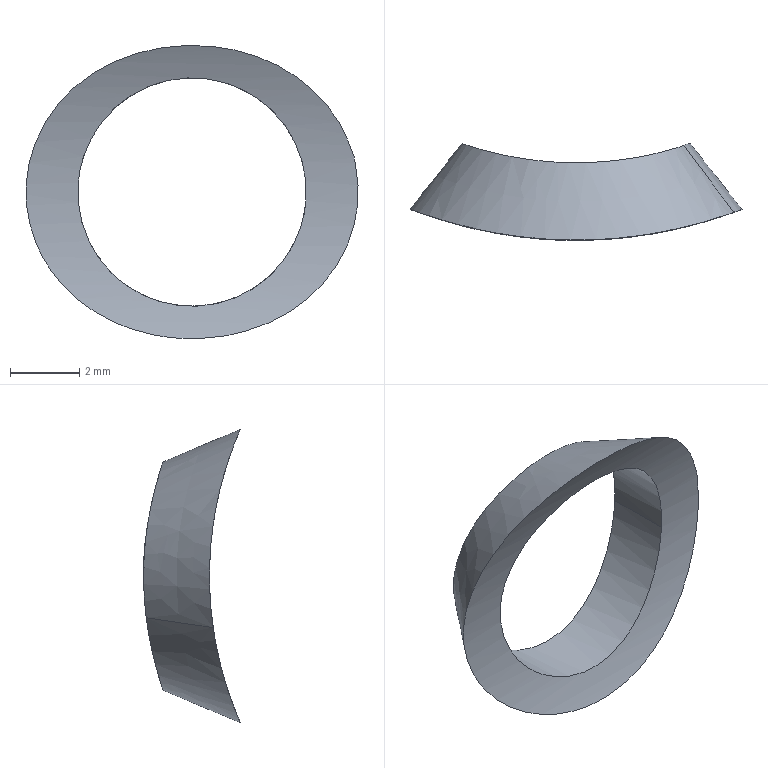Part | STEP file | 2026.6.15-Main Assembly图.sldasm-Part-181 | 1 solid | 5 faces | box 9.599 x 2.798 x 8.476 mm | volume 26.852 mm3 | cylinder 3 | spline 2 | commonest cylinder face diameters 6.6 x2 21 x1
STEP:
#1=CARTESIAN_POINT('',(-1619.46,1436.593,3406.881));
#2=VERTEX_POINT('',#1);
#3=CARTESIAN_POINT('',(-1620.893,1434.658,3406.596));
#4=VERTEX_POINT('',#3);
#5=CARTESIAN_POINT('',(-1619.46,1436.593,3406.881));
#6=CARTESIAN_POINT('',(-1620.893,1434.658,3406.596));
#7=B_SPLINE_CURVE_WITH_KNOTS('',1,(#5,#6),.UNSPECIFIED.,.F.,.F.,(2,2),(0.,1.),.UNSPECIFIED.);
#8=EDGE_CURVE('',#2,#4,#7,.T.);
#9=ORIENTED_EDGE('',*,*,#8,.T.);
#10=CARTESIAN_POINT('',(-1611.83,1434.677,3409.435));
#11=VERTEX_POINT('',#10);
#12=CARTESIAN_POINT('',(-1620.893,1434.658,3406.596));
#13=CARTESIAN_POINT('',(-1621.008,1434.698,3406.877));
#14=CARTESIAN_POINT('',(-1621.09,1434.728,3407.166));
#15=CARTESIAN_POINT('',(-1621.186,1434.764,3407.762));
#16=CARTESIAN_POINT('',(-1621.2,1434.769,3408.071));
#17=CARTESIAN_POINT('',(-1621.167,1434.756,3408.522));
#18=CARTESIAN_POINT('',(-1621.147,1434.749,3408.671));
#19=CARTESIAN_POINT('',(-1621.09,1434.728,3408.968));
#20=CARTESIAN_POINT('',(-1621.053,1434.715,3409.117));
#21=CARTESIAN_POINT('',(-1620.917,1434.666,3409.549));
#22=CARTESIAN_POINT('',(-1620.795,1434.623,3409.823));
#23=CARTESIAN_POINT('',(-1620.491,1434.523,3410.341));
#24=CARTESIAN_POINT('',(-1620.311,1434.466,3410.581));
#25=CARTESIAN_POINT('',(-1619.908,1434.35,3411.017));
#26=CARTESIAN_POINT('',(-1619.682,1434.289,3411.216));
#27=CARTESIAN_POINT('',(-1619.198,1434.174,3411.562));
#28=CARTESIAN_POINT('',(-1618.941,1434.12,3411.711));
#29=CARTESIAN_POINT('',(-1618.396,1434.024,3411.962));
#30=CARTESIAN_POINT('',(-1618.111,1433.982,3412.064));
#31=CARTESIAN_POINT('',(-1617.531,1433.918,3412.217));
#32=CARTESIAN_POINT('',(-1617.234,1433.895,3412.27));
#33=CARTESIAN_POINT('',(-1616.627,1433.87,3412.327));
#34=CARTESIAN_POINT('',(-1616.324,1433.868,3412.332));
#35=CARTESIAN_POINT('',(-1615.723,1433.885,3412.293));
#36=CARTESIAN_POINT('',(-1615.423,1433.904,3412.25));
#37=CARTESIAN_POINT('',(-1614.832,1433.961,3412.115));
#38=CARTESIAN_POINT('',(-1614.547,1433.999,3412.024));
#39=CARTESIAN_POINT('',(-1613.999,1434.089,3411.794));
#40=CARTESIAN_POINT('',(-1613.733,1434.141,3411.654));
#41=CARTESIAN_POINT('',(-1613.234,1434.254,3411.325));
#42=CARTESIAN_POINT('',(-1613.004,1434.313,3411.139));
#43=CARTESIAN_POINT('',(-1612.69,1434.401,3410.828));
#44=CARTESIAN_POINT('',(-1612.59,1434.43,3410.718));
#45=CARTESIAN_POINT('',(-1612.402,1434.487,3410.487));
#46=CARTESIAN_POINT('',(-1612.313,1434.515,3410.365));
#47=CARTESIAN_POINT('',(-1612.068,1434.594,3409.988));
#48=CARTESIAN_POINT('',(-1611.933,1434.64,3409.721));
#49=CARTESIAN_POINT('',(-1611.83,1434.677,3409.435));
#50=B_SPLINE_CURVE_WITH_KNOTS('',3,(#12,#13,#14,#15,#16,#17,#18,#19,#20,#21,#22,#23,#24,#25,#26,#27,#28,#29,#30,#31,#32,#33,#34,#35,#36,#37,#38,#39,#40,#41,#42,#43,#44,#45,#46,#47,#48,#49),.UNSPECIFIED.,.F.,.F.,(4,2,2,2,2,2,2,2,2,2,2,2,2,2,2,2,2,2,4),(0.,0.0009051,0.00181,0.002263,0.002715,0.003621,0.004526,0.005431,0.006336,0.007241,0.008146,0.009051,0.009956,0.01086,0.01177,0.01267,0.01312,0.01358,0.01448),.UNSPECIFIED.);
#51=EDGE_CURVE('',#4,#11,#50,.T.);
#52=ORIENTED_EDGE('',*,*,#51,.T.);
#53=CARTESIAN_POINT('',(-1613.274,1436.605,3409.178));
#54=VERTEX_POINT('',#53);
#55=CARTESIAN_POINT('',(-1613.274,1436.605,3409.178));
#56=CARTESIAN_POINT('',(-1611.83,1434.677,3409.435));
#57=B_SPLINE_CURVE_WITH_KNOTS('',1,(#55,#56),.UNSPECIFIED.,.F.,.F.,(2,2),(0.,1.),.UNSPECIFIED.);
#58=EDGE_CURVE('',#54,#11,#57,.T.);
#59=ORIENTED_EDGE('',*,*,#58,.F.);
#60=CARTESIAN_POINT('',(-1619.678,1436.666,3408.345));
#61=VERTEX_POINT('',#60);
#62=CARTESIAN_POINT('',(-1613.274,1436.605,3409.178));
#63=CARTESIAN_POINT('',(-1613.4,1436.567,3409.536));
#64=CARTESIAN_POINT('',(-1613.58,1436.509,3409.86));
#65=CARTESIAN_POINT('',(-1614.051,1436.382,3410.446));
#66=CARTESIAN_POINT('',(-1614.329,1436.316,3410.692));
#67=CARTESIAN_POINT('',(-1614.97,1436.201,3411.09));
#68=CARTESIAN_POINT('',(-1615.315,1436.157,3411.23));
#69=CARTESIAN_POINT('',(-1616.059,1436.105,3411.392));
#70=CARTESIAN_POINT('',(-1616.435,1436.1,3411.408));
#71=CARTESIAN_POINT('',(-1617.002,1436.124,3411.334));
#72=CARTESIAN_POINT('',(-1617.186,1436.136,3411.294));
#73=CARTESIAN_POINT('',(-1617.544,1436.171,3411.183));
#74=CARTESIAN_POINT('',(-1617.719,1436.193,3411.112));
#75=CARTESIAN_POINT('',(-1618.054,1436.244,3410.941));
#76=CARTESIAN_POINT('',(-1618.212,1436.273,3410.843));
#77=CARTESIAN_POINT('',(-1618.51,1436.334,3410.62));
#78=CARTESIAN_POINT('',(-1618.652,1436.366,3410.495));
#79=CARTESIAN_POINT('',(-1618.909,1436.43,3410.225));
#80=CARTESIAN_POINT('',(-1619.025,1436.462,3410.08));
#81=CARTESIAN_POINT('',(-1619.232,1436.522,3409.771));
#82=CARTESIAN_POINT('',(-1619.324,1436.55,3409.606));
#83=CARTESIAN_POINT('',(-1619.477,1436.598,3409.263));
#84=CARTESIAN_POINT('',(-1619.539,1436.619,3409.086));
#85=CARTESIAN_POINT('',(-1619.632,1436.65,3408.723));
#86=CARTESIAN_POINT('',(-1619.663,1436.661,3408.536));
#87=CARTESIAN_POINT('',(-1619.678,1436.666,3408.345));
#88=B_SPLINE_CURVE_WITH_KNOTS('',3,(#62,#63,#64,#65,#66,#67,#68,#69,#70,#71,#72,#73,#74,#75,#76,#77,#78,#79,#80,#81,#82,#83,#84,#85,#86,#87),.UNSPECIFIED.,.F.,.F.,(4,2,2,2,2,2,2,2,2,2,2,2,4),(0.,0.001127,0.002254,0.003381,0.004507,0.005071,0.005634,0.006198,0.006761,0.007325,0.007888,0.008452,0.009015),.UNSPECIFIED.);
#89=EDGE_CURVE('',#54,#61,#88,.T.);
#90=ORIENTED_EDGE('',*,*,#89,.T.);
#91=CARTESIAN_POINT('',(-1619.678,1436.666,3408.345));
#92=CARTESIAN_POINT('',(-1619.698,1436.673,3408.095));
#93=CARTESIAN_POINT('',(-1619.689,1436.669,3407.847));
#94=CARTESIAN_POINT('',(-1619.616,1436.645,3407.357));
#95=CARTESIAN_POINT('',(-1619.551,1436.622,3407.113));
#96=CARTESIAN_POINT('',(-1619.46,1436.593,3406.881));
#97=B_SPLINE_CURVE_WITH_KNOTS('',3,(#91,#92,#93,#94,#95,#96),.UNSPECIFIED.,.F.,.F.,(4,2,4),(0.,0.000743,0.001486),.UNSPECIFIED.);
#98=EDGE_CURVE('',#61,#2,#97,.T.);
#99=ORIENTED_EDGE('',*,*,#98,.T.);
#100=EDGE_LOOP('',(#9,#52,#59,#90,#99));
#101=FACE_OUTER_BOUND('',#100,.T.);
#102=CARTESIAN_POINT('',(-1611.815,1434.657,3409.437));
#103=CARTESIAN_POINT('',(-1611.869,1434.638,3409.585));
#104=CARTESIAN_POINT('',(-1611.899,1434.628,3409.657));
#105=CARTESIAN_POINT('',(-1612.032,1434.582,3409.934));
#106=CARTESIAN_POINT('',(-1612.106,1434.557,3410.068));
#107=CARTESIAN_POINT('',(-1612.268,1434.505,3410.324));
#108=CARTESIAN_POINT('',(-1612.355,1434.477,3410.447));
#109=CARTESIAN_POINT('',(-1612.543,1434.42,3410.683));
#110=CARTESIAN_POINT('',(-1612.643,1434.39,3410.797));
#111=CARTESIAN_POINT('',(-1612.958,1434.301,3411.116));
#112=CARTESIAN_POINT('',(-1613.185,1434.243,3411.302));
#113=CARTESIAN_POINT('',(-1613.548,1434.159,3411.548));
#114=CARTESIAN_POINT('',(-1613.673,1434.132,3411.624));
#115=CARTESIAN_POINT('',(-1613.931,1434.081,3411.765));
#116=CARTESIAN_POINT('',(-1614.061,1434.056,3411.828));
#117=CARTESIAN_POINT('',(-1614.458,1433.989,3412.002));
#118=CARTESIAN_POINT('',(-1614.729,1433.951,3412.094));
#119=CARTESIAN_POINT('',(-1615.147,1433.907,3412.199));
#120=CARTESIAN_POINT('',(-1615.289,1433.894,3412.229));
#121=CARTESIAN_POINT('',(-1615.572,1433.873,3412.277));
#122=CARTESIAN_POINT('',(-1615.713,1433.865,3412.296));
#123=CARTESIAN_POINT('',(-1615.996,1433.854,3412.322));
#124=CARTESIAN_POINT('',(-1616.137,1433.85,3412.33));
#125=CARTESIAN_POINT('',(-1616.422,1433.848,3412.335));
#126=CARTESIAN_POINT('',(-1616.565,1433.849,3412.333));
#127=CARTESIAN_POINT('',(-1616.996,1433.86,3412.309));
#128=CARTESIAN_POINT('',(-1617.278,1433.876,3412.272));
#129=CARTESIAN_POINT('',(-1617.697,1433.914,3412.184));
#130=CARTESIAN_POINT('',(-1617.836,1433.928,3412.149));
#131=CARTESIAN_POINT('',(-1618.114,1433.962,3412.067));
#132=CARTESIAN_POINT('',(-1618.251,1433.981,3412.02));
#133=CARTESIAN_POINT('',(-1618.655,1434.044,3411.863));
#134=CARTESIAN_POINT('',(-1618.915,1434.092,3411.737));
#135=CARTESIAN_POINT('',(-1619.29,1434.173,3411.508));
#136=CARTESIAN_POINT('',(-1619.413,1434.201,3411.425));
#137=CARTESIAN_POINT('',(-1619.648,1434.258,3411.249));
#138=CARTESIAN_POINT('',(-1619.762,1434.288,3411.155));
#139=CARTESIAN_POINT('',(-1619.979,1434.346,3410.955));
#140=CARTESIAN_POINT('',(-1620.083,1434.376,3410.85));
#141=CARTESIAN_POINT('',(-1620.282,1434.434,3410.626));
#142=CARTESIAN_POINT('',(-1620.376,1434.463,3410.508));
#143=CARTESIAN_POINT('',(-1620.641,1434.547,3410.134));
#144=CARTESIAN_POINT('',(-1620.789,1434.597,3409.867));
#145=CARTESIAN_POINT('',(-1620.965,1434.659,3409.439));
#146=CARTESIAN_POINT('',(-1621.016,1434.677,3409.292));
#147=CARTESIAN_POINT('',(-1621.101,1434.707,3408.989));
#148=CARTESIAN_POINT('',(-1621.135,1434.72,3408.833));
#149=CARTESIAN_POINT('',(-1621.206,1434.746,3408.364));
#150=CARTESIAN_POINT('',(-1621.216,1434.75,3408.048));
#151=CARTESIAN_POINT('',(-1621.18,1434.736,3407.655));
#152=CARTESIAN_POINT('',(-1621.171,1434.733,3407.576));
#153=CARTESIAN_POINT('',(-1621.147,1434.724,3407.419));
#154=CARTESIAN_POINT('',(-1621.132,1434.719,3407.341));
#155=CARTESIAN_POINT('',(-1621.082,1434.701,3407.108));
#156=CARTESIAN_POINT('',(-1621.04,1434.685,3406.957));
#157=CARTESIAN_POINT('',(-1620.888,1434.631,3406.516));
#158=CARTESIAN_POINT('',(-1620.754,1434.585,3406.239));
#159=CARTESIAN_POINT('',(-1620.427,1434.478,3405.718));
#160=CARTESIAN_POINT('',(-1620.239,1434.42,3405.484));
#161=CARTESIAN_POINT('',(-1619.926,1434.332,3405.166));
#162=CARTESIAN_POINT('',(-1619.817,1434.302,3405.066));
#163=CARTESIAN_POINT('',(-1619.589,1434.244,3404.877));
#164=CARTESIAN_POINT('',(-1619.47,1434.215,3404.788));
#165=CARTESIAN_POINT('',(-1619.106,1434.131,3404.542));
#166=CARTESIAN_POINT('',(-1618.851,1434.08,3404.404));
#167=CARTESIAN_POINT('',(-1618.454,1434.012,3404.23));
#168=CARTESIAN_POINT('',(-1618.318,1433.991,3404.177));
#169=CARTESIAN_POINT('',(-1618.043,1433.953,3404.084));
#170=CARTESIAN_POINT('',(-1617.906,1433.936,3404.043));
#171=CARTESIAN_POINT('',(-1617.49,1433.892,3403.938));
#172=CARTESIAN_POINT('',(-1617.21,1433.871,3403.891));
#173=CARTESIAN_POINT('',(-1616.782,1433.854,3403.851));
#174=CARTESIAN_POINT('',(-1616.637,1433.85,3403.843));
#175=CARTESIAN_POINT('',(-1616.352,1433.848,3403.837));
#176=CARTESIAN_POINT('',(-1616.21,1433.849,3403.84));
#177=CARTESIAN_POINT('',(-1615.927,1433.856,3403.856));
#178=CARTESIAN_POINT('',(-1615.785,1433.862,3403.869));
#179=CARTESIAN_POINT('',(-1615.502,1433.878,3403.906));
#180=CARTESIAN_POINT('',(-1615.359,1433.888,3403.93));
#181=CARTESIAN_POINT('',(-1614.937,1433.926,3404.019));
#182=CARTESIAN_POINT('',(-1614.662,1433.96,3404.1));
#183=CARTESIAN_POINT('',(-1614.258,1434.022,3404.256));
#184=CARTESIAN_POINT('',(-1614.125,1434.045,3404.315));
#185=CARTESIAN_POINT('',(-1613.862,1434.094,3404.444));
#186=CARTESIAN_POINT('',(-1613.734,1434.119,3404.514));
#187=CARTESIAN_POINT('',(-1613.362,1434.2,3404.741));
#188=CARTESIAN_POINT('',(-1613.126,1434.258,3404.916));
#189=CARTESIAN_POINT('',(-1612.797,1434.347,3405.218));
#190=CARTESIAN_POINT('',(-1612.691,1434.376,3405.325));
#191=CARTESIAN_POINT('',(-1612.493,1434.435,3405.549));
#192=CARTESIAN_POINT('',(-1612.4,1434.463,3405.666));
#193=CARTESIAN_POINT('',(-1612.225,1434.518,3405.912));
#194=CARTESIAN_POINT('',(-1612.144,1434.545,3406.04));
#195=CARTESIAN_POINT('',(-1612.033,1434.582,3406.241));
#196=CARTESIAN_POINT('',(-1611.998,1434.594,3406.31));
#197=CARTESIAN_POINT('',(-1611.93,1434.617,3406.45));
#198=CARTESIAN_POINT('',(-1611.899,1434.628,3406.521));
#199=CARTESIAN_POINT('',(-1611.75,1434.68,3406.882));
#200=CARTESIAN_POINT('',(-1611.666,1434.711,3407.183));
#201=CARTESIAN_POINT('',(-1611.594,1434.737,3407.649));
#202=CARTESIAN_POINT('',(-1611.58,1434.743,3407.807));
#203=CARTESIAN_POINT('',(-1611.57,1434.746,3408.126));
#204=CARTESIAN_POINT('',(-1611.575,1434.744,3408.286));
#205=CARTESIAN_POINT('',(-1611.618,1434.728,3408.759));
#206=CARTESIAN_POINT('',(-1611.685,1434.704,3409.067));
#207=CARTESIAN_POINT('',(-1611.685,1434.704,3409.067));
#208=CARTESIAN_POINT('',(-1611.762,1434.676,3409.29));
#209=CARTESIAN_POINT('',(-1611.815,1434.657,3409.437));
#210=CARTESIAN_POINT('',(-1613.275,1436.606,3409.178));
#211=CARTESIAN_POINT('',(-1613.316,1436.593,3409.296));
#212=CARTESIAN_POINT('',(-1613.339,1436.586,3409.354));
#213=CARTESIAN_POINT('',(-1613.441,1436.554,3409.575));
#214=CARTESIAN_POINT('',(-1613.497,1436.536,3409.681));
#215=CARTESIAN_POINT('',(-1613.618,1436.5,3409.883));
#216=CARTESIAN_POINT('',(-1613.683,1436.482,3409.98));
#217=CARTESIAN_POINT('',(-1613.822,1436.443,3410.164));
#218=CARTESIAN_POINT('',(-1613.895,1436.424,3410.252));
#219=CARTESIAN_POINT('',(-1614.124,1436.366,3410.497));
#220=CARTESIAN_POINT('',(-1614.286,1436.329,3410.638));
#221=CARTESIAN_POINT('',(-1614.539,1436.278,3410.821));
#222=CARTESIAN_POINT('',(-1614.625,1436.262,3410.878));
#223=CARTESIAN_POINT('',(-1614.801,1436.232,3410.981));
#224=CARTESIAN_POINT('',(-1614.889,1436.218,3411.028));
#225=CARTESIAN_POINT('',(-1615.154,1436.181,3411.153));
#226=CARTESIAN_POINT('',(-1615.332,1436.16,3411.218));
#227=CARTESIAN_POINT('',(-1615.602,1436.137,3411.293));
#228=CARTESIAN_POINT('',(-1615.693,1436.13,3411.314));
#229=CARTESIAN_POINT('',(-1615.873,1436.12,3411.347));
#230=CARTESIAN_POINT('',(-1615.963,1436.115,3411.36));
#231=CARTESIAN_POINT('',(-1616.141,1436.11,3411.378));
#232=CARTESIAN_POINT('',(-1616.23,1436.108,3411.384));
#233=CARTESIAN_POINT('',(-1616.409,1436.107,3411.387));
#234=CARTESIAN_POINT('',(-1616.499,1436.107,3411.386));
#235=CARTESIAN_POINT('',(-1616.771,1436.113,3411.369));
#236=CARTESIAN_POINT('',(-1616.949,1436.121,3411.344));
#237=CARTESIAN_POINT('',(-1617.218,1436.14,3411.282));
#238=CARTESIAN_POINT('',(-1617.308,1436.148,3411.257));
#239=CARTESIAN_POINT('',(-1617.489,1436.166,3411.199));
#240=CARTESIAN_POINT('',(-1617.579,1436.177,3411.166));
#241=CARTESIAN_POINT('',(-1617.846,1436.211,3411.053));
#242=CARTESIAN_POINT('',(-1618.022,1436.239,3410.961));
#243=CARTESIAN_POINT('',(-1618.28,1436.287,3410.792));
#244=CARTESIAN_POINT('',(-1618.366,1436.304,3410.73));
#245=CARTESIAN_POINT('',(-1618.532,1436.339,3410.597));
#246=CARTESIAN_POINT('',(-1618.613,1436.358,3410.526));
#247=CARTESIAN_POINT('',(-1618.769,1436.395,3410.374));
#248=CARTESIAN_POINT('',(-1618.845,1436.414,3410.293));
#249=CARTESIAN_POINT('',(-1618.99,1436.453,3410.119));
#250=CARTESIAN_POINT('',(-1619.06,1436.472,3410.027));
#251=CARTESIAN_POINT('',(-1619.257,1436.529,3409.734));
#252=CARTESIAN_POINT('',(-1619.37,1436.564,3409.522));
#253=CARTESIAN_POINT('',(-1619.504,1436.607,3409.179));
#254=CARTESIAN_POINT('',(-1619.544,1436.62,3409.061));
#255=CARTESIAN_POINT('',(-1619.609,1436.642,3408.817));
#256=CARTESIAN_POINT('',(-1619.635,1436.651,3408.691));
#257=CARTESIAN_POINT('',(-1619.69,1436.67,3408.312));
#258=CARTESIAN_POINT('',(-1619.698,1436.673,3408.055));
#259=CARTESIAN_POINT('',(-1619.67,1436.663,3407.736));
#260=CARTESIAN_POINT('',(-1619.663,1436.661,3407.673));
#261=CARTESIAN_POINT('',(-1619.644,1436.654,3407.546));
#262=CARTESIAN_POINT('',(-1619.633,1436.65,3407.482));
#263=CARTESIAN_POINT('',(-1619.594,1436.637,3407.295));
#264=CARTESIAN_POINT('',(-1619.562,1436.626,3407.173));
#265=CARTESIAN_POINT('',(-1619.445,1436.588,3406.819));
#266=CARTESIAN_POINT('',(-1619.343,1436.555,3406.597));
#267=CARTESIAN_POINT('',(-1619.097,1436.482,3406.187));
#268=CARTESIAN_POINT('',(-1618.958,1436.443,3406.004));
#269=CARTESIAN_POINT('',(-1618.731,1436.386,3405.76));
#270=CARTESIAN_POINT('',(-1618.653,1436.367,3405.683));
#271=CARTESIAN_POINT('',(-1618.49,1436.33,3405.54));
#272=CARTESIAN_POINT('',(-1618.406,1436.312,3405.473));
#273=CARTESIAN_POINT('',(-1618.152,1436.261,3405.289));
#274=CARTESIAN_POINT('',(-1617.979,1436.231,3405.188));
#275=CARTESIAN_POINT('',(-1617.713,1436.193,3405.062));
#276=CARTESIAN_POINT('',(-1617.623,1436.182,3405.024));
#277=CARTESIAN_POINT('',(-1617.443,1436.161,3404.958));
#278=CARTESIAN_POINT('',(-1617.353,1436.152,3404.929));
#279=CARTESIAN_POINT('',(-1617.085,1436.129,3404.855));
#280=CARTESIAN_POINT('',(-1616.907,1436.118,3404.822));
#281=CARTESIAN_POINT('',(-1616.636,1436.11,3404.794));
#282=CARTESIAN_POINT('',(-1616.545,1436.108,3404.789));
#283=CARTESIAN_POINT('',(-1616.366,1436.107,3404.785));
#284=CARTESIAN_POINT('',(-1616.276,1436.107,3404.787));
#285=CARTESIAN_POINT('',(-1616.098,1436.111,3404.798));
#286=CARTESIAN_POINT('',(-1616.008,1436.114,3404.807));
#287=CARTESIAN_POINT('',(-1615.829,1436.122,3404.833));
#288=CARTESIAN_POINT('',(-1615.738,1436.127,3404.85));
#289=CARTESIAN_POINT('',(-1615.467,1436.147,3404.912));
#290=CARTESIAN_POINT('',(-1615.288,1436.165,3404.969));
#291=CARTESIAN_POINT('',(-1615.021,1436.199,3405.081));
#292=CARTESIAN_POINT('',(-1614.932,1436.212,3405.123));
#293=CARTESIAN_POINT('',(-1614.754,1436.24,3405.217));
#294=CARTESIAN_POINT('',(-1614.667,1436.255,3405.269));
#295=CARTESIAN_POINT('',(-1614.41,1436.303,3405.437));
#296=CARTESIAN_POINT('',(-1614.244,1436.338,3405.568));
#297=CARTESIAN_POINT('',(-1614.007,1436.395,3405.799));
#298=CARTESIAN_POINT('',(-1613.93,1436.415,3405.882));
#299=CARTESIAN_POINT('',(-1613.785,1436.453,3406.055));
#300=CARTESIAN_POINT('',(-1613.716,1436.472,3406.147));
#301=CARTESIAN_POINT('',(-1613.586,1436.51,3406.339));
#302=CARTESIAN_POINT('',(-1613.525,1436.528,3406.441));
#303=CARTESIAN_POINT('',(-1613.441,1436.554,3406.6));
#304=CARTESIAN_POINT('',(-1613.414,1436.562,3406.655));
#305=CARTESIAN_POINT('',(-1613.363,1436.578,3406.766));
#306=CARTESIAN_POINT('',(-1613.339,1436.586,3406.823));
#307=CARTESIAN_POINT('',(-1613.226,1436.622,3407.112));
#308=CARTESIAN_POINT('',(-1613.16,1436.645,3407.355));
#309=CARTESIAN_POINT('',(-1613.105,1436.664,3407.732));
#310=CARTESIAN_POINT('',(-1613.094,1436.668,3407.86));
#311=CARTESIAN_POINT('',(-1613.086,1436.67,3408.118));
#312=CARTESIAN_POINT('',(-1613.09,1436.669,3408.248));
#313=CARTESIAN_POINT('',(-1613.123,1436.657,3408.631));
#314=CARTESIAN_POINT('',(-1613.175,1436.639,3408.88));
#315=CARTESIAN_POINT('',(-1613.175,1436.639,3408.88));
#316=CARTESIAN_POINT('',(-1613.234,1436.62,3409.059));
#317=CARTESIAN_POINT('',(-1613.275,1436.606,3409.178));
#318=CARTESIAN_POINT('',(-1613.304,1436.645,3409.173));
#319=CARTESIAN_POINT('',(-1613.345,1436.632,3409.29));
#320=CARTESIAN_POINT('',(-1613.368,1436.625,3409.348));
#321=CARTESIAN_POINT('',(-1613.469,1436.593,3409.568));
#322=CARTESIAN_POINT('',(-1613.524,1436.576,3409.673));
#323=CARTESIAN_POINT('',(-1613.645,1436.54,3409.874));
#324=CARTESIAN_POINT('',(-1613.71,1436.522,3409.97));
#325=CARTESIAN_POINT('',(-1613.847,1436.484,3410.153));
#326=CARTESIAN_POINT('',(-1613.921,1436.464,3410.241));
#327=CARTESIAN_POINT('',(-1614.147,1436.407,3410.485));
#328=CARTESIAN_POINT('',(-1614.308,1436.371,3410.625));
#329=CARTESIAN_POINT('',(-1614.559,1436.321,3410.807));
#330=CARTESIAN_POINT('',(-1614.644,1436.305,3410.863));
#331=CARTESIAN_POINT('',(-1614.818,1436.275,3410.966));
#332=CARTESIAN_POINT('',(-1614.906,1436.262,3411.012));
#333=CARTESIAN_POINT('',(-1615.168,1436.224,3411.136));
#334=CARTESIAN_POINT('',(-1615.344,1436.204,3411.201));
#335=CARTESIAN_POINT('',(-1615.611,1436.181,3411.275));
#336=CARTESIAN_POINT('',(-1615.701,1436.175,3411.295));
#337=CARTESIAN_POINT('',(-1615.879,1436.164,3411.329));
#338=CARTESIAN_POINT('',(-1615.968,1436.16,3411.341));
#339=CARTESIAN_POINT('',(-1616.144,1436.155,3411.359));
#340=CARTESIAN_POINT('',(-1616.232,1436.153,3411.365));
#341=CARTESIAN_POINT('',(-1616.409,1436.152,3411.369));
#342=CARTESIAN_POINT('',(-1616.498,1436.152,3411.367));
#343=CARTESIAN_POINT('',(-1616.766,1436.158,3411.35));
#344=CARTESIAN_POINT('',(-1616.943,1436.166,3411.325));
#345=CARTESIAN_POINT('',(-1617.208,1436.185,3411.264));
#346=CARTESIAN_POINT('',(-1617.297,1436.192,3411.239));
#347=CARTESIAN_POINT('',(-1617.476,1436.21,3411.182));
#348=CARTESIAN_POINT('',(-1617.565,1436.22,3411.149));
#349=CARTESIAN_POINT('',(-1617.83,1436.254,3411.037));
#350=CARTESIAN_POINT('',(-1618.004,1436.282,3410.946));
#351=CARTESIAN_POINT('',(-1618.26,1436.329,3410.778));
#352=CARTESIAN_POINT('',(-1618.345,1436.346,3410.716));
#353=CARTESIAN_POINT('',(-1618.51,1436.381,3410.584));
#354=CARTESIAN_POINT('',(-1618.59,1436.399,3410.514));
#355=CARTESIAN_POINT('',(-1618.745,1436.436,3410.362));
#356=CARTESIAN_POINT('',(-1618.82,1436.455,3410.282));
#357=CARTESIAN_POINT('',(-1618.964,1436.493,3410.109));
#358=CARTESIAN_POINT('',(-1619.034,1436.512,3410.017));
#359=CARTESIAN_POINT('',(-1619.23,1436.569,3409.726));
#360=CARTESIAN_POINT('',(-1619.341,1436.603,3409.515));
#361=CARTESIAN_POINT('',(-1619.475,1436.646,3409.174));
#362=CARTESIAN_POINT('',(-1619.514,1436.659,3409.056));
#363=CARTESIAN_POINT('',(-1619.579,1436.681,3408.814));
#364=CARTESIAN_POINT('',(-1619.605,1436.69,3408.688));
#365=CARTESIAN_POINT('',(-1619.66,1436.708,3408.311));
#366=CARTESIAN_POINT('',(-1619.668,1436.711,3408.055));
#367=CARTESIAN_POINT('',(-1619.64,1436.702,3407.738));
#368=CARTESIAN_POINT('',(-1619.633,1436.699,3407.675));
#369=CARTESIAN_POINT('',(-1619.614,1436.693,3407.548));
#370=CARTESIAN_POINT('',(-1619.603,1436.689,3407.485));
#371=CARTESIAN_POINT('',(-1619.565,1436.676,3407.299));
#372=CARTESIAN_POINT('',(-1619.532,1436.665,3407.177));
#373=CARTESIAN_POINT('',(-1619.416,1436.627,3406.825));
#374=CARTESIAN_POINT('',(-1619.315,1436.595,3406.605));
#375=CARTESIAN_POINT('',(-1619.071,1436.522,3406.196));
#376=CARTESIAN_POINT('',(-1618.932,1436.484,3406.014));
#377=CARTESIAN_POINT('',(-1618.707,1436.427,3405.771));
#378=CARTESIAN_POINT('',(-1618.629,1436.408,3405.696));
#379=CARTESIAN_POINT('',(-1618.468,1436.372,3405.553));
#380=CARTESIAN_POINT('',(-1618.385,1436.354,3405.487));
#381=CARTESIAN_POINT('',(-1618.133,1436.304,3405.304));
#382=CARTESIAN_POINT('',(-1617.961,1436.275,3405.204));
#383=CARTESIAN_POINT('',(-1617.698,1436.237,3405.079));
#384=CARTESIAN_POINT('',(-1617.609,1436.226,3405.041));
#385=CARTESIAN_POINT('',(-1617.431,1436.205,3404.975));
#386=CARTESIAN_POINT('',(-1617.342,1436.197,3404.947));
#387=CARTESIAN_POINT('',(-1617.076,1436.174,3404.874));
#388=CARTESIAN_POINT('',(-1616.9,1436.163,3404.841));
#389=CARTESIAN_POINT('',(-1616.633,1436.155,3404.813));
#390=CARTESIAN_POINT('',(-1616.543,1436.153,3404.808));
#391=CARTESIAN_POINT('',(-1616.366,1436.152,3404.804));
#392=CARTESIAN_POINT('',(-1616.278,1436.152,3404.806));
#393=CARTESIAN_POINT('',(-1616.101,1436.156,3404.817));
#394=CARTESIAN_POINT('',(-1616.013,1436.159,3404.826));
#395=CARTESIAN_POINT('',(-1615.835,1436.167,3404.851));
#396=CARTESIAN_POINT('',(-1615.745,1436.172,3404.868));
#397=CARTESIAN_POINT('',(-1615.477,1436.191,3404.93));
#398=CARTESIAN_POINT('',(-1615.301,1436.209,3404.986));
#399=CARTESIAN_POINT('',(-1615.036,1436.243,3405.098));
#400=CARTESIAN_POINT('',(-1614.948,1436.255,3405.14));
#401=CARTESIAN_POINT('',(-1614.772,1436.283,3405.233));
#402=CARTESIAN_POINT('',(-1614.686,1436.298,3405.284));
#403=CARTESIAN_POINT('',(-1614.431,1436.345,3405.451));
#404=CARTESIAN_POINT('',(-1614.266,1436.38,3405.581));
#405=CARTESIAN_POINT('',(-1614.031,1436.436,3405.811));
#406=CARTESIAN_POINT('',(-1613.955,1436.456,3405.893));
#407=CARTESIAN_POINT('',(-1613.811,1436.494,3406.065));
#408=CARTESIAN_POINT('',(-1613.742,1436.513,3406.156));
#409=CARTESIAN_POINT('',(-1613.613,1436.55,3406.348));
#410=CARTESIAN_POINT('',(-1613.553,1436.568,3406.449));
#411=CARTESIAN_POINT('',(-1613.469,1436.593,3406.607));
#412=CARTESIAN_POINT('',(-1613.443,1436.601,3406.662));
#413=CARTESIAN_POINT('',(-1613.392,1436.617,3406.772));
#414=CARTESIAN_POINT('',(-1613.368,1436.625,3406.829));
#415=CARTESIAN_POINT('',(-1613.255,1436.661,3407.116));
#416=CARTESIAN_POINT('',(-1613.19,1436.683,3407.358));
#417=CARTESIAN_POINT('',(-1613.135,1436.702,3407.734));
#418=CARTESIAN_POINT('',(-1613.124,1436.706,3407.861));
#419=CARTESIAN_POINT('',(-1613.116,1436.709,3408.118));
#420=CARTESIAN_POINT('',(-1613.12,1436.707,3408.247));
#421=CARTESIAN_POINT('',(-1613.154,1436.696,3408.628));
#422=CARTESIAN_POINT('',(-1613.205,1436.678,3408.877));
#423=CARTESIAN_POINT('',(-1613.205,1436.678,3408.877));
#424=CARTESIAN_POINT('',(-1613.264,1436.659,3409.055));
#425=CARTESIAN_POINT('',(-1613.304,1436.645,3409.173));
#426=B_SPLINE_SURFACE_WITH_KNOTS('',1,3,((#102,#103,#104,#105,#106,#107,#108,#109,#110,#111,#112,#113,#114,#115,#116,#117,#118,#119,#120,#121,#122,#123,#124,#125,#126,#127,#128,#129,#130,#131,#132,#133,#134,#135,#136,#137,#138,#139,#140,#141,#142,#143,#144,#145,#146,#147,#148,#149,#150,#151,#152,#153,#154,#155,#156,#157,#158,#159,#160,#161,#162,#163,#164,#165,#166,#167,#168,#169,#170,#171,#172,#173,#174,#175,#176,#177,#178,#179,#180,#181,#182,#183,#184,#185,#186,#187,#188,#189,#190,#191,#192,#193,#194,#195,#196,#197,#198,#199,#200,#201,#202,#203,#204,#205,#206,#207,#208,#209),(#210,#211,#212,#213,#214,#215,#216,#217,#218,#219,#220,#221,#222,#223,#224,#225,#226,#227,#228,#229,#230,#231,#232,#233,#234,#235,#236,#237,#238,#239,#240,#241,#242,#243,#244,#245,#246,#247,#248,#249,#250,#251,#252,#253,#254,#255,#256,#257,#258,#259,#260,#261,#262,#263,#264,#265,#266,#267,#268,#269,#270,#271,#272,#273,#274,#275,#276,#277,#278,#279,#280,#281,#282,#283,#284,#285,#286,#287,#288,#289,#290,#291,#292,#293,#294,#295,#296,#297,#298,#299,#300,#301,#302,#303,#304,#305,#306,#307,#308,#309,#310,#311,#312,#313,#314,#315,#316,#317),(#318,#319,#320,#321,#322,#323,#324,#325,#326,#327,#328,#329,#330,#331,#332,#333,#334,#335,#336,#337,#338,#339,#340,#341,#342,#343,#344,#345,#346,#347,#348,#349,#350,#351,#352,#353,#354,#355,#356,#357,#358,#359,#360,#361,#362,#363,#364,#365,#366,#367,#368,#369,#370,#371,#372,#373,#374,#375,#376,#377,#378,#379,#380,#381,#382,#383,#384,#385,#386,#387,#388,#389,#390,#391,#392,#393,#394,#395,#396,#397,#398,#399,#400,#401,#402,#403,#404,#405,#406,#407,#408,#409,#410,#411,#412,#413,#414,#415,#416,#417,#418,#419,#420,#421,#422,#423,#424,#425)),.UNSPECIFIED.,.F.,.T.,.F.,(2,1,2),(4,2,2,2,2,2,2,2,2,2,2,2,2,2,2,2,2,2,2,2,2,2,2,2,2,2,2,2,2,2,2,2,2,2,2,2,2,2,2,2,2,2,2,2,2,2,2,2,2,2,2,2,2,4),(0.,0.9804,1.),(0.,0.01538,0.03077,0.04615,0.06154,0.09231,0.1077,0.1231,0.1538,0.1692,0.1846,0.2,0.2154,0.2462,0.2615,0.2769,0.3077,0.3231,0.3385,0.3538,0.3692,0.4,0.4154,0.4308,0.4615,0.4692,0.4769,0.4923,0.5231,0.5538,0.5692,0.5846,0.6154,0.6308,0.6462,0.6769,0.6923,0.7077,0.7231,0.7385,0.7692,0.7846,0.8,0.8308,0.8462,0.8615,0.8769,0.8846,0.8923,0.9231,0.9385,0.9538,0.9846,1.),.UNSPECIFIED.);
#427=ADVANCED_FACE('',(#101),#426,.T.);
#428=CARTESIAN_POINT('',(-1619.678,1434.761,3408.345));
#429=VERTEX_POINT('',#428);
#430=CARTESIAN_POINT('',(-1619.678,1439.564,3408.345));
#431=DIRECTION('',(0.,1.,0.));
#432=VECTOR('',#431,1000.);
#433=LINE('',#430,#432);
#434=EDGE_CURVE('',#429,#61,#433,.T.);
#435=ORIENTED_EDGE('',*,*,#434,.F.);
#436=CARTESIAN_POINT('',(-1613.098,1434.761,3407.827));
#437=VERTEX_POINT('',#436);
#438=CARTESIAN_POINT('',(-1619.678,1434.761,3408.345));
#439=CARTESIAN_POINT('',(-1619.695,1434.767,3408.127));
#440=CARTESIAN_POINT('',(-1619.691,1434.765,3407.91));
#441=CARTESIAN_POINT('',(-1619.639,1434.749,3407.481));
#442=CARTESIAN_POINT('',(-1619.592,1434.734,3407.265));
#443=CARTESIAN_POINT('',(-1619.457,1434.694,3406.854));
#444=CARTESIAN_POINT('',(-1619.371,1434.668,3406.657));
#445=CARTESIAN_POINT('',(-1619.159,1434.61,3406.281));
#446=CARTESIAN_POINT('',(-1619.034,1434.577,3406.103));
#447=CARTESIAN_POINT('',(-1618.617,1434.475,3405.616));
#448=CARTESIAN_POINT('',(-1618.272,1434.402,3405.343));
#449=CARTESIAN_POINT('',(-1617.7,1434.316,3405.051));
#450=CARTESIAN_POINT('',(-1617.496,1434.292,3404.97));
#451=CARTESIAN_POINT('',(-1617.079,1434.254,3404.852));
#452=CARTESIAN_POINT('',(-1616.867,1434.241,3404.814));
#453=CARTESIAN_POINT('',(-1616.435,1434.23,3404.78));
#454=CARTESIAN_POINT('',(-1616.213,1434.231,3404.784));
#455=CARTESIAN_POINT('',(-1615.783,1434.248,3404.835));
#456=CARTESIAN_POINT('',(-1615.572,1434.263,3404.881));
#457=CARTESIAN_POINT('',(-1615.158,1434.306,3405.016));
#458=CARTESIAN_POINT('',(-1614.96,1434.332,3405.104));
#459=CARTESIAN_POINT('',(-1614.586,1434.392,3405.314));
#460=CARTESIAN_POINT('',(-1614.408,1434.426,3405.438));
#461=CARTESIAN_POINT('',(-1614.081,1434.495,3405.718));
#462=CARTESIAN_POINT('',(-1613.933,1434.529,3405.871));
#463=CARTESIAN_POINT('',(-1613.667,1434.596,3406.208));
#464=CARTESIAN_POINT('',(-1613.548,1434.628,3406.392));
#465=CARTESIAN_POINT('',(-1613.353,1434.684,3406.774));
#466=CARTESIAN_POINT('',(-1613.274,1434.707,3406.974));
#467=CARTESIAN_POINT('',(-1613.155,1434.743,3407.392));
#468=CARTESIAN_POINT('',(-1613.116,1434.756,3407.609));
#469=CARTESIAN_POINT('',(-1613.098,1434.761,3407.827));
#470=B_SPLINE_CURVE_WITH_KNOTS('',3,(#438,#439,#440,#441,#442,#443,#444,#445,#446,#447,#448,#449,#450,#451,#452,#453,#454,#455,#456,#457,#458,#459,#460,#461,#462,#463,#464,#465,#466,#467,#468,#469),.UNSPECIFIED.,.F.,.F.,(4,2,2,2,2,2,2,2,2,2,2,2,2,2,2,4),(0.,0.0006488,0.001298,0.001946,0.002595,0.003893,0.004541,0.00519,0.005839,0.006488,0.007136,0.007785,0.008434,0.009083,0.009732,0.01038),.UNSPECIFIED.);
#471=EDGE_CURVE('',#429,#437,#470,.T.);
#472=ORIENTED_EDGE('',*,*,#471,.T.);
#473=CARTESIAN_POINT('',(-1613.098,1436.666,3407.827));
#474=VERTEX_POINT('',#473);
#475=CARTESIAN_POINT('',(-1613.098,1439.564,3407.827));
#476=DIRECTION('',(0.,1.,0.));
#477=VECTOR('',#476,1000.);
#478=LINE('',#475,#477);
#479=EDGE_CURVE('',#437,#474,#478,.T.);
#480=ORIENTED_EDGE('',*,*,#479,.T.);
#481=CARTESIAN_POINT('',(-1619.46,1436.593,3406.881));
#482=CARTESIAN_POINT('',(-1619.324,1436.549,3406.533));
#483=CARTESIAN_POINT('',(-1619.129,1436.489,3406.212));
#484=CARTESIAN_POINT('',(-1618.772,1436.395,3405.797));
#485=CARTESIAN_POINT('',(-1618.641,1436.364,3405.668));
#486=CARTESIAN_POINT('',(-1618.358,1436.301,3405.432));
#487=CARTESIAN_POINT('',(-1618.206,1436.272,3405.326));
#488=CARTESIAN_POINT('',(-1617.889,1436.218,3405.141));
#489=CARTESIAN_POINT('',(-1617.723,1436.194,3405.062));
#490=CARTESIAN_POINT('',(-1617.375,1436.153,3404.932));
#491=CARTESIAN_POINT('',(-1617.194,1436.137,3404.881));
#492=CARTESIAN_POINT('',(-1616.826,1436.115,3404.81));
#493=CARTESIAN_POINT('',(-1616.639,1436.108,3404.791));
#494=CARTESIAN_POINT('',(-1616.268,1436.106,3404.783));
#495=CARTESIAN_POINT('',(-1616.083,1436.11,3404.795));
#496=CARTESIAN_POINT('',(-1615.527,1436.136,3404.879));
#497=CARTESIAN_POINT('',(-1615.175,1436.174,3404.995));
#498=CARTESIAN_POINT('',(-1614.517,1436.277,3405.343));
#499=CARTESIAN_POINT('',(-1614.225,1436.34,3405.567));
#500=CARTESIAN_POINT('',(-1613.722,1436.468,3406.108));
#501=CARTESIAN_POINT('',(-1613.519,1436.529,3406.414));
#502=CARTESIAN_POINT('',(-1613.219,1436.624,3407.095));
#503=CARTESIAN_POINT('',(-1613.128,1436.656,3407.452));
#504=CARTESIAN_POINT('',(-1613.098,1436.666,3407.827));
#505=B_SPLINE_CURVE_WITH_KNOTS('',3,(#481,#482,#483,#484,#485,#486,#487,#488,#489,#490,#491,#492,#493,#494,#495,#496,#497,#498,#499,#500,#501,#502,#503,#504),.UNSPECIFIED.,.F.,.F.,(4,2,2,2,2,2,2,2,2,2,2,4),(0.,0.001123,0.001684,0.002246,0.002807,0.003368,0.00393,0.004491,0.005614,0.006737,0.00786,0.008983),.UNSPECIFIED.);
#506=EDGE_CURVE('',#2,#474,#505,.T.);
#507=ORIENTED_EDGE('',*,*,#506,.F.);
#508=ORIENTED_EDGE('',*,*,#98,.F.);
#509=EDGE_LOOP('',(#435,#472,#480,#507,#508));
#510=FACE_OUTER_BOUND('',#509,.T.);
#511=CARTESIAN_POINT('',(-1616.388,1439.564,3408.086));
#512=DIRECTION('',(0.,1.,0.));
#513=DIRECTION('',(-0.9969,0.,0.0785));
#514=AXIS2_PLACEMENT_3D('',#511,#512,#513);
#515=CYLINDRICAL_SURFACE('',#514,3.3);
#516=ADVANCED_FACE('',(#510),#515,.F.);
#517=CARTESIAN_POINT('',(-1611.83,1434.677,3409.435));
#518=CARTESIAN_POINT('',(-1611.805,1434.686,3409.364));
#519=CARTESIAN_POINT('',(-1611.78,1434.695,3409.294));
#520=CARTESIAN_POINT('',(-1611.742,1434.706,3409.188));
#521=CARTESIAN_POINT('',(-1611.729,1434.71,3409.153));
#522=CARTESIAN_POINT('',(-1611.713,1434.714,3409.109));
#523=CARTESIAN_POINT('',(-1611.71,1434.715,3409.1));
#524=CARTESIAN_POINT('',(-1611.703,1434.717,3409.083));
#525=CARTESIAN_POINT('',(-1611.699,1434.718,3409.074));
#526=CARTESIAN_POINT('',(-1611.693,1434.72,3409.047));
#527=CARTESIAN_POINT('',(-1611.69,1434.722,3409.029));
#528=CARTESIAN_POINT('',(-1611.659,1434.736,3408.866));
#529=CARTESIAN_POINT('',(-1611.636,1434.746,3408.72));
#530=CARTESIAN_POINT('',(-1611.583,1434.767,3408.279));
#531=CARTESIAN_POINT('',(-1611.579,1434.768,3407.982));
#532=CARTESIAN_POINT('',(-1611.638,1434.746,3407.398));
#533=CARTESIAN_POINT('',(-1611.702,1434.722,3407.106));
#534=CARTESIAN_POINT('',(-1611.89,1434.655,3406.552));
#535=CARTESIAN_POINT('',(-1612.013,1434.612,3406.289));
#536=CARTESIAN_POINT('',(-1612.469,1434.463,3405.538));
#537=CARTESIAN_POINT('',(-1612.878,1434.34,3405.109));
#538=CARTESIAN_POINT('',(-1613.83,1434.115,3404.435));
#539=CARTESIAN_POINT('',(-1614.371,1434.015,3404.188));
#540=CARTESIAN_POINT('',(-1615.513,1433.888,3403.884));
#541=CARTESIAN_POINT('',(-1616.112,1433.861,3403.824));
#542=CARTESIAN_POINT('',(-1617.296,1433.889,3403.89));
#543=CARTESIAN_POINT('',(-1617.884,1433.946,3404.015));
#544=CARTESIAN_POINT('',(-1618.975,1434.118,3404.452));
#545=CARTESIAN_POINT('',(-1619.479,1434.234,3404.765));
#546=CARTESIAN_POINT('',(-1620.326,1434.465,3405.564));
#547=CARTESIAN_POINT('',(-1620.669,1434.58,3406.051));
#548=CARTESIAN_POINT('',(-1620.893,1434.658,3406.596));
#549=B_SPLINE_CURVE_WITH_KNOTS('',3,(#517,#518,#519,#520,#521,#522,#523,#524,#525,#526,#527,#528,#529,#530,#531,#532,#533,#534,#535,#536,#537,#538,#539,#540,#541,#542,#543,#544,#545,#546,#547,#548),.UNSPECIFIED.,.F.,.F.,(4,2,2,2,2,2,2,2,2,2,2,2,2,2,2,4),(0.,0.0002257,0.0003385,0.0003667,0.000395,0.0004514,0.0009028,0.001806,0.002708,0.003611,0.005417,0.007222,0.009028,0.01083,0.01264,0.01444),.UNSPECIFIED.);
#550=EDGE_CURVE('',#11,#4,#549,.T.);
#551=ORIENTED_EDGE('',*,*,#550,.F.);
#552=ORIENTED_EDGE('',*,*,#51,.F.);
#553=EDGE_LOOP('',(#551,#552));
#554=FACE_OUTER_BOUND('',#553,.T.);
#555=CARTESIAN_POINT('',(-1613.098,1434.761,3407.827));
#556=CARTESIAN_POINT('',(-1613.081,1434.767,3408.046));
#557=CARTESIAN_POINT('',(-1613.086,1434.765,3408.263));
#558=CARTESIAN_POINT('',(-1613.137,1434.749,3408.692));
#559=CARTESIAN_POINT('',(-1613.185,1434.734,3408.907));
#560=CARTESIAN_POINT('',(-1613.319,1434.694,3409.319));
#561=CARTESIAN_POINT('',(-1613.406,1434.668,3409.515));
#562=CARTESIAN_POINT('',(-1613.617,1434.61,3409.891));
#563=CARTESIAN_POINT('',(-1613.742,1434.577,3410.07));
#564=CARTESIAN_POINT('',(-1614.159,1434.475,3410.557));
#565=CARTESIAN_POINT('',(-1614.504,1434.402,3410.829));
#566=CARTESIAN_POINT('',(-1615.077,1434.316,3411.122));
#567=CARTESIAN_POINT('',(-1615.28,1434.292,3411.202));
#568=CARTESIAN_POINT('',(-1615.698,1434.254,3411.321));
#569=CARTESIAN_POINT('',(-1615.91,1434.241,3411.359));
#570=CARTESIAN_POINT('',(-1616.342,1434.23,3411.393));
#571=CARTESIAN_POINT('',(-1616.563,1434.231,3411.389));
#572=CARTESIAN_POINT('',(-1616.993,1434.248,3411.338));
#573=CARTESIAN_POINT('',(-1617.204,1434.263,3411.291));
#574=CARTESIAN_POINT('',(-1617.618,1434.306,3411.156));
#575=CARTESIAN_POINT('',(-1617.816,1434.332,3411.069));
#576=CARTESIAN_POINT('',(-1618.191,1434.392,3410.859));
#577=CARTESIAN_POINT('',(-1618.369,1434.426,3410.735));
#578=CARTESIAN_POINT('',(-1618.696,1434.495,3410.455));
#579=CARTESIAN_POINT('',(-1618.844,1434.529,3410.301));
#580=CARTESIAN_POINT('',(-1619.11,1434.596,3409.965));
#581=CARTESIAN_POINT('',(-1619.228,1434.628,3409.781));
#582=CARTESIAN_POINT('',(-1619.424,1434.684,3409.399));
#583=CARTESIAN_POINT('',(-1619.503,1434.707,3409.199));
#584=CARTESIAN_POINT('',(-1619.622,1434.743,3408.781));
#585=CARTESIAN_POINT('',(-1619.661,1434.756,3408.564));
#586=CARTESIAN_POINT('',(-1619.678,1434.761,3408.345));
#587=B_SPLINE_CURVE_WITH_KNOTS('',3,(#555,#556,#557,#558,#559,#560,#561,#562,#563,#564,#565,#566,#567,#568,#569,#570,#571,#572,#573,#574,#575,#576,#577,#578,#579,#580,#581,#582,#583,#584,#585,#586),.UNSPECIFIED.,.F.,.F.,(4,2,2,2,2,2,2,2,2,2,2,2,2,2,2,4),(0.,0.0006488,0.001298,0.001946,0.002595,0.003893,0.004541,0.00519,0.005839,0.006488,0.007136,0.007785,0.008434,0.009083,0.009732,0.01038),.UNSPECIFIED.);
#588=EDGE_CURVE('',#437,#429,#587,.T.);
#589=ORIENTED_EDGE('',*,*,#588,.F.);
#590=ORIENTED_EDGE('',*,*,#471,.F.);
#591=EDGE_LOOP('',(#589,#590));
#592=FACE_BOUND('',#591,.T.);
#593=CARTESIAN_POINT('',(-1621.788,1424.264,3408.086));
#594=DIRECTION('',(-1.,0.,0.));
#595=DIRECTION('',(0.,0.,-1.));
#596=AXIS2_PLACEMENT_3D('',#593,#594,#595);
#597=CYLINDRICAL_SURFACE('',#596,10.5);
#598=ADVANCED_FACE('',(#554,#592),#597,.F.);
#599=ORIENTED_EDGE('',*,*,#588,.T.);
#600=ORIENTED_EDGE('',*,*,#434,.T.);
#601=ORIENTED_EDGE('',*,*,#89,.F.);
#602=CARTESIAN_POINT('',(-1613.098,1436.666,3407.827));
#603=CARTESIAN_POINT('',(-1613.08,1436.672,3408.057));
#604=CARTESIAN_POINT('',(-1613.086,1436.668,3408.284));
#605=CARTESIAN_POINT('',(-1613.13,1436.656,3408.624));
#606=CARTESIAN_POINT('',(-1613.151,1436.653,3408.737));
#607=CARTESIAN_POINT('',(-1613.181,1436.652,3408.863));
#608=CARTESIAN_POINT('',(-1613.184,1436.652,3408.877));
#609=CARTESIAN_POINT('',(-1613.191,1436.646,3408.905));
#610=CARTESIAN_POINT('',(-1613.202,1436.638,3408.946));
#611=CARTESIAN_POINT('',(-1613.213,1436.631,3408.987));
#612=CARTESIAN_POINT('',(-1613.237,1436.618,3409.069));
#613=CARTESIAN_POINT('',(-1613.255,1436.611,3409.124));
#614=CARTESIAN_POINT('',(-1613.274,1436.605,3409.178));
#615=B_SPLINE_CURVE_WITH_KNOTS('',3,(#602,#603,#604,#605,#606,#607,#608,#609,#610,#611,#612,#613,#614),.UNSPECIFIED.,.F.,.F.,(4,2,2,2,1,2,4),(0.,0.0006835,0.001025,0.001068,0.001111,0.001196,0.001367),.UNSPECIFIED.);
#616=EDGE_CURVE('',#474,#54,#615,.T.);
#617=ORIENTED_EDGE('',*,*,#616,.F.);
#618=ORIENTED_EDGE('',*,*,#479,.F.);
#619=EDGE_LOOP('',(#599,#600,#601,#617,#618));
#620=FACE_OUTER_BOUND('',#619,.T.);
#621=CARTESIAN_POINT('',(-1616.388,1439.564,3408.086));
#622=DIRECTION('',(0.,1.,0.));
#623=DIRECTION('',(-0.9969,0.,0.0785));
#624=AXIS2_PLACEMENT_3D('',#621,#622,#623);
#625=CYLINDRICAL_SURFACE('',#624,3.3);
#626=ADVANCED_FACE('',(#620),#625,.F.);
#627=ORIENTED_EDGE('',*,*,#550,.T.);
#628=ORIENTED_EDGE('',*,*,#8,.F.);
#629=ORIENTED_EDGE('',*,*,#506,.T.);
#630=ORIENTED_EDGE('',*,*,#616,.T.);
#631=ORIENTED_EDGE('',*,*,#58,.T.);
#632=EDGE_LOOP('',(#627,#628,#629,#630,#631));
#633=FACE_OUTER_BOUND('',#632,.T.);
#634=CARTESIAN_POINT('',(-1611.815,1434.657,3409.437));
#635=CARTESIAN_POINT('',(-1611.869,1434.638,3409.585));
#636=CARTESIAN_POINT('',(-1611.899,1434.628,3409.657));
#637=CARTESIAN_POINT('',(-1612.032,1434.582,3409.934));
#638=CARTESIAN_POINT('',(-1612.106,1434.557,3410.068));
#639=CARTESIAN_POINT('',(-1612.268,1434.505,3410.324));
#640=CARTESIAN_POINT('',(-1612.355,1434.477,3410.447));
#641=CARTESIAN_POINT('',(-1612.543,1434.42,3410.683));
#642=CARTESIAN_POINT('',(-1612.643,1434.39,3410.797));
#643=CARTESIAN_POINT('',(-1612.958,1434.301,3411.116));
#644=CARTESIAN_POINT('',(-1613.185,1434.243,3411.302));
#645=CARTESIAN_POINT('',(-1613.548,1434.159,3411.548));
#646=CARTESIAN_POINT('',(-1613.673,1434.132,3411.624));
#647=CARTESIAN_POINT('',(-1613.931,1434.081,3411.765));
#648=CARTESIAN_POINT('',(-1614.061,1434.056,3411.828));
#649=CARTESIAN_POINT('',(-1614.458,1433.989,3412.002));
#650=CARTESIAN_POINT('',(-1614.729,1433.951,3412.094));
#651=CARTESIAN_POINT('',(-1615.147,1433.907,3412.199));
#652=CARTESIAN_POINT('',(-1615.289,1433.894,3412.229));
#653=CARTESIAN_POINT('',(-1615.572,1433.873,3412.277));
#654=CARTESIAN_POINT('',(-1615.713,1433.865,3412.296));
#655=CARTESIAN_POINT('',(-1615.996,1433.854,3412.322));
#656=CARTESIAN_POINT('',(-1616.137,1433.85,3412.33));
#657=CARTESIAN_POINT('',(-1616.422,1433.848,3412.335));
#658=CARTESIAN_POINT('',(-1616.565,1433.849,3412.333));
#659=CARTESIAN_POINT('',(-1616.996,1433.86,3412.309));
#660=CARTESIAN_POINT('',(-1617.278,1433.876,3412.272));
#661=CARTESIAN_POINT('',(-1617.697,1433.914,3412.184));
#662=CARTESIAN_POINT('',(-1617.836,1433.928,3412.149));
#663=CARTESIAN_POINT('',(-1618.114,1433.962,3412.067));
#664=CARTESIAN_POINT('',(-1618.251,1433.981,3412.02));
#665=CARTESIAN_POINT('',(-1618.655,1434.044,3411.863));
#666=CARTESIAN_POINT('',(-1618.915,1434.092,3411.737));
#667=CARTESIAN_POINT('',(-1619.29,1434.173,3411.508));
#668=CARTESIAN_POINT('',(-1619.413,1434.201,3411.425));
#669=CARTESIAN_POINT('',(-1619.648,1434.258,3411.249));
#670=CARTESIAN_POINT('',(-1619.762,1434.288,3411.155));
#671=CARTESIAN_POINT('',(-1619.979,1434.346,3410.955));
#672=CARTESIAN_POINT('',(-1620.083,1434.376,3410.85));
#673=CARTESIAN_POINT('',(-1620.282,1434.434,3410.626));
#674=CARTESIAN_POINT('',(-1620.376,1434.463,3410.508));
#675=CARTESIAN_POINT('',(-1620.641,1434.547,3410.134));
#676=CARTESIAN_POINT('',(-1620.789,1434.597,3409.867));
#677=CARTESIAN_POINT('',(-1620.965,1434.659,3409.439));
#678=CARTESIAN_POINT('',(-1621.016,1434.677,3409.292));
#679=CARTESIAN_POINT('',(-1621.101,1434.707,3408.989));
#680=CARTESIAN_POINT('',(-1621.135,1434.72,3408.833));
#681=CARTESIAN_POINT('',(-1621.206,1434.746,3408.364));
#682=CARTESIAN_POINT('',(-1621.216,1434.75,3408.048));
#683=CARTESIAN_POINT('',(-1621.18,1434.736,3407.655));
#684=CARTESIAN_POINT('',(-1621.171,1434.733,3407.576));
#685=CARTESIAN_POINT('',(-1621.147,1434.724,3407.419));
#686=CARTESIAN_POINT('',(-1621.132,1434.719,3407.341));
#687=CARTESIAN_POINT('',(-1621.082,1434.701,3407.108));
#688=CARTESIAN_POINT('',(-1621.04,1434.685,3406.957));
#689=CARTESIAN_POINT('',(-1620.888,1434.631,3406.516));
#690=CARTESIAN_POINT('',(-1620.754,1434.585,3406.239));
#691=CARTESIAN_POINT('',(-1620.427,1434.478,3405.718));
#692=CARTESIAN_POINT('',(-1620.239,1434.42,3405.484));
#693=CARTESIAN_POINT('',(-1619.926,1434.332,3405.166));
#694=CARTESIAN_POINT('',(-1619.817,1434.302,3405.066));
#695=CARTESIAN_POINT('',(-1619.589,1434.244,3404.877));
#696=CARTESIAN_POINT('',(-1619.47,1434.215,3404.788));
#697=CARTESIAN_POINT('',(-1619.106,1434.131,3404.542));
#698=CARTESIAN_POINT('',(-1618.851,1434.08,3404.404));
#699=CARTESIAN_POINT('',(-1618.454,1434.012,3404.23));
#700=CARTESIAN_POINT('',(-1618.318,1433.991,3404.177));
#701=CARTESIAN_POINT('',(-1618.043,1433.953,3404.084));
#702=CARTESIAN_POINT('',(-1617.906,1433.936,3404.043));
#703=CARTESIAN_POINT('',(-1617.49,1433.892,3403.938));
#704=CARTESIAN_POINT('',(-1617.21,1433.871,3403.891));
#705=CARTESIAN_POINT('',(-1616.782,1433.854,3403.851));
#706=CARTESIAN_POINT('',(-1616.637,1433.85,3403.843));
#707=CARTESIAN_POINT('',(-1616.352,1433.848,3403.837));
#708=CARTESIAN_POINT('',(-1616.21,1433.849,3403.84));
#709=CARTESIAN_POINT('',(-1615.927,1433.856,3403.856));
#710=CARTESIAN_POINT('',(-1615.785,1433.862,3403.869));
#711=CARTESIAN_POINT('',(-1615.502,1433.878,3403.906));
#712=CARTESIAN_POINT('',(-1615.359,1433.888,3403.93));
#713=CARTESIAN_POINT('',(-1614.937,1433.926,3404.019));
#714=CARTESIAN_POINT('',(-1614.662,1433.96,3404.1));
#715=CARTESIAN_POINT('',(-1614.258,1434.022,3404.256));
#716=CARTESIAN_POINT('',(-1614.125,1434.045,3404.315));
#717=CARTESIAN_POINT('',(-1613.862,1434.094,3404.444));
#718=CARTESIAN_POINT('',(-1613.734,1434.119,3404.514));
#719=CARTESIAN_POINT('',(-1613.362,1434.2,3404.741));
#720=CARTESIAN_POINT('',(-1613.126,1434.258,3404.916));
#721=CARTESIAN_POINT('',(-1612.797,1434.347,3405.218));
#722=CARTESIAN_POINT('',(-1612.691,1434.376,3405.325));
#723=CARTESIAN_POINT('',(-1612.493,1434.435,3405.549));
#724=CARTESIAN_POINT('',(-1612.4,1434.463,3405.666));
#725=CARTESIAN_POINT('',(-1612.225,1434.518,3405.912));
#726=CARTESIAN_POINT('',(-1612.144,1434.545,3406.04));
#727=CARTESIAN_POINT('',(-1612.033,1434.582,3406.241));
#728=CARTESIAN_POINT('',(-1611.998,1434.594,3406.31));
#729=CARTESIAN_POINT('',(-1611.93,1434.617,3406.45));
#730=CARTESIAN_POINT('',(-1611.899,1434.628,3406.521));
#731=CARTESIAN_POINT('',(-1611.75,1434.68,3406.882));
#732=CARTESIAN_POINT('',(-1611.666,1434.711,3407.183));
#733=CARTESIAN_POINT('',(-1611.594,1434.737,3407.649));
#734=CARTESIAN_POINT('',(-1611.58,1434.743,3407.807));
#735=CARTESIAN_POINT('',(-1611.57,1434.746,3408.126));
#736=CARTESIAN_POINT('',(-1611.575,1434.744,3408.286));
#737=CARTESIAN_POINT('',(-1611.618,1434.728,3408.759));
#738=CARTESIAN_POINT('',(-1611.685,1434.704,3409.067));
#739=CARTESIAN_POINT('',(-1611.685,1434.704,3409.067));
#740=CARTESIAN_POINT('',(-1611.762,1434.676,3409.29));
#741=CARTESIAN_POINT('',(-1611.815,1434.657,3409.437));
#742=CARTESIAN_POINT('',(-1613.275,1436.606,3409.178));
#743=CARTESIAN_POINT('',(-1613.316,1436.593,3409.296));
#744=CARTESIAN_POINT('',(-1613.339,1436.586,3409.354));
#745=CARTESIAN_POINT('',(-1613.441,1436.554,3409.575));
#746=CARTESIAN_POINT('',(-1613.497,1436.536,3409.681));
#747=CARTESIAN_POINT('',(-1613.618,1436.5,3409.883));
#748=CARTESIAN_POINT('',(-1613.683,1436.482,3409.98));
#749=CARTESIAN_POINT('',(-1613.822,1436.443,3410.164));
#750=CARTESIAN_POINT('',(-1613.895,1436.424,3410.252));
#751=CARTESIAN_POINT('',(-1614.124,1436.366,3410.497));
#752=CARTESIAN_POINT('',(-1614.286,1436.329,3410.638));
#753=CARTESIAN_POINT('',(-1614.539,1436.278,3410.821));
#754=CARTESIAN_POINT('',(-1614.625,1436.262,3410.878));
#755=CARTESIAN_POINT('',(-1614.801,1436.232,3410.981));
#756=CARTESIAN_POINT('',(-1614.889,1436.218,3411.028));
#757=CARTESIAN_POINT('',(-1615.154,1436.181,3411.153));
#758=CARTESIAN_POINT('',(-1615.332,1436.16,3411.218));
#759=CARTESIAN_POINT('',(-1615.602,1436.137,3411.293));
#760=CARTESIAN_POINT('',(-1615.693,1436.13,3411.314));
#761=CARTESIAN_POINT('',(-1615.873,1436.12,3411.347));
#762=CARTESIAN_POINT('',(-1615.963,1436.115,3411.36));
#763=CARTESIAN_POINT('',(-1616.141,1436.11,3411.378));
#764=CARTESIAN_POINT('',(-1616.23,1436.108,3411.384));
#765=CARTESIAN_POINT('',(-1616.409,1436.107,3411.387));
#766=CARTESIAN_POINT('',(-1616.499,1436.107,3411.386));
#767=CARTESIAN_POINT('',(-1616.771,1436.113,3411.369));
#768=CARTESIAN_POINT('',(-1616.949,1436.121,3411.344));
#769=CARTESIAN_POINT('',(-1617.218,1436.14,3411.282));
#770=CARTESIAN_POINT('',(-1617.308,1436.148,3411.257));
#771=CARTESIAN_POINT('',(-1617.489,1436.166,3411.199));
#772=CARTESIAN_POINT('',(-1617.579,1436.177,3411.166));
#773=CARTESIAN_POINT('',(-1617.846,1436.211,3411.053));
#774=CARTESIAN_POINT('',(-1618.022,1436.239,3410.961));
#775=CARTESIAN_POINT('',(-1618.28,1436.287,3410.792));
#776=CARTESIAN_POINT('',(-1618.366,1436.304,3410.73));
#777=CARTESIAN_POINT('',(-1618.532,1436.339,3410.597));
#778=CARTESIAN_POINT('',(-1618.613,1436.358,3410.526));
#779=CARTESIAN_POINT('',(-1618.769,1436.395,3410.374));
#780=CARTESIAN_POINT('',(-1618.845,1436.414,3410.293));
#781=CARTESIAN_POINT('',(-1618.99,1436.453,3410.119));
#782=CARTESIAN_POINT('',(-1619.06,1436.472,3410.027));
#783=CARTESIAN_POINT('',(-1619.257,1436.529,3409.734));
#784=CARTESIAN_POINT('',(-1619.37,1436.564,3409.522));
#785=CARTESIAN_POINT('',(-1619.504,1436.607,3409.179));
#786=CARTESIAN_POINT('',(-1619.544,1436.62,3409.061));
#787=CARTESIAN_POINT('',(-1619.609,1436.642,3408.817));
#788=CARTESIAN_POINT('',(-1619.635,1436.651,3408.691));
#789=CARTESIAN_POINT('',(-1619.69,1436.67,3408.312));
#790=CARTESIAN_POINT('',(-1619.698,1436.673,3408.055));
#791=CARTESIAN_POINT('',(-1619.67,1436.663,3407.736));
#792=CARTESIAN_POINT('',(-1619.663,1436.661,3407.673));
#793=CARTESIAN_POINT('',(-1619.644,1436.654,3407.546));
#794=CARTESIAN_POINT('',(-1619.633,1436.65,3407.482));
#795=CARTESIAN_POINT('',(-1619.594,1436.637,3407.295));
#796=CARTESIAN_POINT('',(-1619.562,1436.626,3407.173));
#797=CARTESIAN_POINT('',(-1619.445,1436.588,3406.819));
#798=CARTESIAN_POINT('',(-1619.343,1436.555,3406.597));
#799=CARTESIAN_POINT('',(-1619.097,1436.482,3406.187));
#800=CARTESIAN_POINT('',(-1618.958,1436.443,3406.004));
#801=CARTESIAN_POINT('',(-1618.731,1436.386,3405.76));
#802=CARTESIAN_POINT('',(-1618.653,1436.367,3405.683));
#803=CARTESIAN_POINT('',(-1618.49,1436.33,3405.54));
#804=CARTESIAN_POINT('',(-1618.406,1436.312,3405.473));
#805=CARTESIAN_POINT('',(-1618.152,1436.261,3405.289));
#806=CARTESIAN_POINT('',(-1617.979,1436.231,3405.188));
#807=CARTESIAN_POINT('',(-1617.713,1436.193,3405.062));
#808=CARTESIAN_POINT('',(-1617.623,1436.182,3405.024));
#809=CARTESIAN_POINT('',(-1617.443,1436.161,3404.958));
#810=CARTESIAN_POINT('',(-1617.353,1436.152,3404.929));
#811=CARTESIAN_POINT('',(-1617.085,1436.129,3404.855));
#812=CARTESIAN_POINT('',(-1616.907,1436.118,3404.822));
#813=CARTESIAN_POINT('',(-1616.636,1436.11,3404.794));
#814=CARTESIAN_POINT('',(-1616.545,1436.108,3404.789));
#815=CARTESIAN_POINT('',(-1616.366,1436.107,3404.785));
#816=CARTESIAN_POINT('',(-1616.276,1436.107,3404.787));
#817=CARTESIAN_POINT('',(-1616.098,1436.111,3404.798));
#818=CARTESIAN_POINT('',(-1616.008,1436.114,3404.807));
#819=CARTESIAN_POINT('',(-1615.829,1436.122,3404.833));
#820=CARTESIAN_POINT('',(-1615.738,1436.127,3404.85));
#821=CARTESIAN_POINT('',(-1615.467,1436.147,3404.912));
#822=CARTESIAN_POINT('',(-1615.288,1436.165,3404.969));
#823=CARTESIAN_POINT('',(-1615.021,1436.199,3405.081));
#824=CARTESIAN_POINT('',(-1614.932,1436.212,3405.123));
#825=CARTESIAN_POINT('',(-1614.754,1436.24,3405.217));
#826=CARTESIAN_POINT('',(-1614.667,1436.255,3405.269));
#827=CARTESIAN_POINT('',(-1614.41,1436.303,3405.437));
#828=CARTESIAN_POINT('',(-1614.244,1436.338,3405.568));
#829=CARTESIAN_POINT('',(-1614.007,1436.395,3405.799));
#830=CARTESIAN_POINT('',(-1613.93,1436.415,3405.882));
#831=CARTESIAN_POINT('',(-1613.785,1436.453,3406.055));
#832=CARTESIAN_POINT('',(-1613.716,1436.472,3406.147));
#833=CARTESIAN_POINT('',(-1613.586,1436.51,3406.339));
#834=CARTESIAN_POINT('',(-1613.525,1436.528,3406.441));
#835=CARTESIAN_POINT('',(-1613.441,1436.554,3406.6));
#836=CARTESIAN_POINT('',(-1613.414,1436.562,3406.655));
#837=CARTESIAN_POINT('',(-1613.363,1436.578,3406.766));
#838=CARTESIAN_POINT('',(-1613.339,1436.586,3406.823));
#839=CARTESIAN_POINT('',(-1613.226,1436.622,3407.112));
#840=CARTESIAN_POINT('',(-1613.16,1436.645,3407.355));
#841=CARTESIAN_POINT('',(-1613.105,1436.664,3407.732));
#842=CARTESIAN_POINT('',(-1613.094,1436.668,3407.86));
#843=CARTESIAN_POINT('',(-1613.086,1436.67,3408.118));
#844=CARTESIAN_POINT('',(-1613.09,1436.669,3408.248));
#845=CARTESIAN_POINT('',(-1613.123,1436.657,3408.631));
#846=CARTESIAN_POINT('',(-1613.175,1436.639,3408.88));
#847=CARTESIAN_POINT('',(-1613.175,1436.639,3408.88));
#848=CARTESIAN_POINT('',(-1613.234,1436.62,3409.059));
#849=CARTESIAN_POINT('',(-1613.275,1436.606,3409.178));
#850=CARTESIAN_POINT('',(-1613.304,1436.645,3409.173));
#851=CARTESIAN_POINT('',(-1613.345,1436.632,3409.29));
#852=CARTESIAN_POINT('',(-1613.368,1436.625,3409.348));
#853=CARTESIAN_POINT('',(-1613.469,1436.593,3409.568));
#854=CARTESIAN_POINT('',(-1613.524,1436.576,3409.673));
#855=CARTESIAN_POINT('',(-1613.645,1436.54,3409.874));
#856=CARTESIAN_POINT('',(-1613.71,1436.522,3409.97));
#857=CARTESIAN_POINT('',(-1613.847,1436.484,3410.153));
#858=CARTESIAN_POINT('',(-1613.921,1436.464,3410.241));
#859=CARTESIAN_POINT('',(-1614.147,1436.407,3410.485));
#860=CARTESIAN_POINT('',(-1614.308,1436.371,3410.625));
#861=CARTESIAN_POINT('',(-1614.559,1436.321,3410.807));
#862=CARTESIAN_POINT('',(-1614.644,1436.305,3410.863));
#863=CARTESIAN_POINT('',(-1614.818,1436.275,3410.966));
#864=CARTESIAN_POINT('',(-1614.906,1436.262,3411.012));
#865=CARTESIAN_POINT('',(-1615.168,1436.224,3411.136));
#866=CARTESIAN_POINT('',(-1615.344,1436.204,3411.201));
#867=CARTESIAN_POINT('',(-1615.611,1436.181,3411.275));
#868=CARTESIAN_POINT('',(-1615.701,1436.175,3411.295));
#869=CARTESIAN_POINT('',(-1615.879,1436.164,3411.329));
#870=CARTESIAN_POINT('',(-1615.968,1436.16,3411.341));
#871=CARTESIAN_POINT('',(-1616.144,1436.155,3411.359));
#872=CARTESIAN_POINT('',(-1616.232,1436.153,3411.365));
#873=CARTESIAN_POINT('',(-1616.409,1436.152,3411.369));
#874=CARTESIAN_POINT('',(-1616.498,1436.152,3411.367));
#875=CARTESIAN_POINT('',(-1616.766,1436.158,3411.35));
#876=CARTESIAN_POINT('',(-1616.943,1436.166,3411.325));
#877=CARTESIAN_POINT('',(-1617.208,1436.185,3411.264));
#878=CARTESIAN_POINT('',(-1617.297,1436.192,3411.239));
#879=CARTESIAN_POINT('',(-1617.476,1436.21,3411.182));
#880=CARTESIAN_POINT('',(-1617.565,1436.22,3411.149));
#881=CARTESIAN_POINT('',(-1617.83,1436.254,3411.037));
#882=CARTESIAN_POINT('',(-1618.004,1436.282,3410.946));
#883=CARTESIAN_POINT('',(-1618.26,1436.329,3410.778));
#884=CARTESIAN_POINT('',(-1618.345,1436.346,3410.716));
#885=CARTESIAN_POINT('',(-1618.51,1436.381,3410.584));
#886=CARTESIAN_POINT('',(-1618.59,1436.399,3410.514));
#887=CARTESIAN_POINT('',(-1618.745,1436.436,3410.362));
#888=CARTESIAN_POINT('',(-1618.82,1436.455,3410.282));
#889=CARTESIAN_POINT('',(-1618.964,1436.493,3410.109));
#890=CARTESIAN_POINT('',(-1619.034,1436.512,3410.017));
#891=CARTESIAN_POINT('',(-1619.23,1436.569,3409.726));
#892=CARTESIAN_POINT('',(-1619.341,1436.603,3409.515));
#893=CARTESIAN_POINT('',(-1619.475,1436.646,3409.174));
#894=CARTESIAN_POINT('',(-1619.514,1436.659,3409.056));
#895=CARTESIAN_POINT('',(-1619.579,1436.681,3408.814));
#896=CARTESIAN_POINT('',(-1619.605,1436.69,3408.688));
#897=CARTESIAN_POINT('',(-1619.66,1436.708,3408.311));
#898=CARTESIAN_POINT('',(-1619.668,1436.711,3408.055));
#899=CARTESIAN_POINT('',(-1619.64,1436.702,3407.738));
#900=CARTESIAN_POINT('',(-1619.633,1436.699,3407.675));
#901=CARTESIAN_POINT('',(-1619.614,1436.693,3407.548));
#902=CARTESIAN_POINT('',(-1619.603,1436.689,3407.485));
#903=CARTESIAN_POINT('',(-1619.565,1436.676,3407.299));
#904=CARTESIAN_POINT('',(-1619.532,1436.665,3407.177));
#905=CARTESIAN_POINT('',(-1619.416,1436.627,3406.825));
#906=CARTESIAN_POINT('',(-1619.315,1436.595,3406.605));
#907=CARTESIAN_POINT('',(-1619.071,1436.522,3406.196));
#908=CARTESIAN_POINT('',(-1618.932,1436.484,3406.014));
#909=CARTESIAN_POINT('',(-1618.707,1436.427,3405.771));
#910=CARTESIAN_POINT('',(-1618.629,1436.408,3405.696));
#911=CARTESIAN_POINT('',(-1618.468,1436.372,3405.553));
#912=CARTESIAN_POINT('',(-1618.385,1436.354,3405.487));
#913=CARTESIAN_POINT('',(-1618.133,1436.304,3405.304));
#914=CARTESIAN_POINT('',(-1617.961,1436.275,3405.204));
#915=CARTESIAN_POINT('',(-1617.698,1436.237,3405.079));
#916=CARTESIAN_POINT('',(-1617.609,1436.226,3405.041));
#917=CARTESIAN_POINT('',(-1617.431,1436.205,3404.975));
#918=CARTESIAN_POINT('',(-1617.342,1436.197,3404.947));
#919=CARTESIAN_POINT('',(-1617.076,1436.174,3404.874));
#920=CARTESIAN_POINT('',(-1616.9,1436.163,3404.841));
#921=CARTESIAN_POINT('',(-1616.633,1436.155,3404.813));
#922=CARTESIAN_POINT('',(-1616.543,1436.153,3404.808));
#923=CARTESIAN_POINT('',(-1616.366,1436.152,3404.804));
#924=CARTESIAN_POINT('',(-1616.278,1436.152,3404.806));
#925=CARTESIAN_POINT('',(-1616.101,1436.156,3404.817));
#926=CARTESIAN_POINT('',(-1616.013,1436.159,3404.826));
#927=CARTESIAN_POINT('',(-1615.835,1436.167,3404.851));
#928=CARTESIAN_POINT('',(-1615.745,1436.172,3404.868));
#929=CARTESIAN_POINT('',(-1615.477,1436.191,3404.93));
#930=CARTESIAN_POINT('',(-1615.301,1436.209,3404.986));
#931=CARTESIAN_POINT('',(-1615.036,1436.243,3405.098));
#932=CARTESIAN_POINT('',(-1614.948,1436.255,3405.14));
#933=CARTESIAN_POINT('',(-1614.772,1436.283,3405.233));
#934=CARTESIAN_POINT('',(-1614.686,1436.298,3405.284));
#935=CARTESIAN_POINT('',(-1614.431,1436.345,3405.451));
#936=CARTESIAN_POINT('',(-1614.266,1436.38,3405.581));
#937=CARTESIAN_POINT('',(-1614.031,1436.436,3405.811));
#938=CARTESIAN_POINT('',(-1613.955,1436.456,3405.893));
#939=CARTESIAN_POINT('',(-1613.811,1436.494,3406.065));
#940=CARTESIAN_POINT('',(-1613.742,1436.513,3406.156));
#941=CARTESIAN_POINT('',(-1613.613,1436.55,3406.348));
#942=CARTESIAN_POINT('',(-1613.553,1436.568,3406.449));
#943=CARTESIAN_POINT('',(-1613.469,1436.593,3406.607));
#944=CARTESIAN_POINT('',(-1613.443,1436.601,3406.662));
#945=CARTESIAN_POINT('',(-1613.392,1436.617,3406.772));
#946=CARTESIAN_POINT('',(-1613.368,1436.625,3406.829));
#947=CARTESIAN_POINT('',(-1613.255,1436.661,3407.116));
#948=CARTESIAN_POINT('',(-1613.19,1436.683,3407.358));
#949=CARTESIAN_POINT('',(-1613.135,1436.702,3407.734));
#950=CARTESIAN_POINT('',(-1613.124,1436.706,3407.861));
#951=CARTESIAN_POINT('',(-1613.116,1436.709,3408.118));
#952=CARTESIAN_POINT('',(-1613.12,1436.707,3408.247));
#953=CARTESIAN_POINT('',(-1613.154,1436.696,3408.628));
#954=CARTESIAN_POINT('',(-1613.205,1436.678,3408.877));
#955=CARTESIAN_POINT('',(-1613.205,1436.678,3408.877));
#956=CARTESIAN_POINT('',(-1613.264,1436.659,3409.055));
#957=CARTESIAN_POINT('',(-1613.304,1436.645,3409.173));
#958=B_SPLINE_SURFACE_WITH_KNOTS('',1,3,((#634,#635,#636,#637,#638,#639,#640,#641,#642,#643,#644,#645,#646,#647,#648,#649,#650,#651,#652,#653,#654,#655,#656,#657,#658,#659,#660,#661,#662,#663,#664,#665,#666,#667,#668,#669,#670,#671,#672,#673,#674,#675,#676,#677,#678,#679,#680,#681,#682,#683,#684,#685,#686,#687,#688,#689,#690,#691,#692,#693,#694,#695,#696,#697,#698,#699,#700,#701,#702,#703,#704,#705,#706,#707,#708,#709,#710,#711,#712,#713,#714,#715,#716,#717,#718,#719,#720,#721,#722,#723,#724,#725,#726,#727,#728,#729,#730,#731,#732,#733,#734,#735,#736,#737,#738,#739,#740,#741),(#742,#743,#744,#745,#746,#747,#748,#749,#750,#751,#752,#753,#754,#755,#756,#757,#758,#759,#760,#761,#762,#763,#764,#765,#766,#767,#768,#769,#770,#771,#772,#773,#774,#775,#776,#777,#778,#779,#780,#781,#782,#783,#784,#785,#786,#787,#788,#789,#790,#791,#792,#793,#794,#795,#796,#797,#798,#799,#800,#801,#802,#803,#804,#805,#806,#807,#808,#809,#810,#811,#812,#813,#814,#815,#816,#817,#818,#819,#820,#821,#822,#823,#824,#825,#826,#827,#828,#829,#830,#831,#832,#833,#834,#835,#836,#837,#838,#839,#840,#841,#842,#843,#844,#845,#846,#847,#848,#849),(#850,#851,#852,#853,#854,#855,#856,#857,#858,#859,#860,#861,#862,#863,#864,#865,#866,#867,#868,#869,#870,#871,#872,#873,#874,#875,#876,#877,#878,#879,#880,#881,#882,#883,#884,#885,#886,#887,#888,#889,#890,#891,#892,#893,#894,#895,#896,#897,#898,#899,#900,#901,#902,#903,#904,#905,#906,#907,#908,#909,#910,#911,#912,#913,#914,#915,#916,#917,#918,#919,#920,#921,#922,#923,#924,#925,#926,#927,#928,#929,#930,#931,#932,#933,#934,#935,#936,#937,#938,#939,#940,#941,#942,#943,#944,#945,#946,#947,#948,#949,#950,#951,#952,#953,#954,#955,#956,#957)),.UNSPECIFIED.,.F.,.T.,.F.,(2,1,2),(4,2,2,2,2,2,2,2,2,2,2,2,2,2,2,2,2,2,2,2,2,2,2,2,2,2,2,2,2,2,2,2,2,2,2,2,2,2,2,2,2,2,2,2,2,2,2,2,2,2,2,2,2,4),(0.,0.9804,1.),(0.,0.01538,0.03077,0.04615,0.06154,0.09231,0.1077,0.1231,0.1538,0.1692,0.1846,0.2,0.2154,0.2462,0.2615,0.2769,0.3077,0.3231,0.3385,0.3538,0.3692,0.4,0.4154,0.4308,0.4615,0.4692,0.4769,0.4923,0.5231,0.5538,0.5692,0.5846,0.6154,0.6308,0.6462,0.6769,0.6923,0.7077,0.7231,0.7385,0.7692,0.7846,0.8,0.8308,0.8462,0.8615,0.8769,0.8846,0.8923,0.9231,0.9385,0.9538,0.9846,1.),.UNSPECIFIED.);
#959=ADVANCED_FACE('',(#633),#958,.T.);
#960=CLOSED_SHELL('',(#427,#516,#598,#626,#959));
#961=MANIFOLD_SOLID_BREP('',#960);
#962=CARTESIAN_POINT('',(0.,0.,0.));
#963=DIRECTION('',(0.,0.,1.));
#964=DIRECTION('',(1.,0.,0.));
#965=AXIS2_PLACEMENT_3D('',#962,#963,#964);
#966=(LENGTH_UNIT()NAMED_UNIT(*)SI_UNIT(.MILLI.,.METRE.));
#967=UNCERTAINTY_MEASURE_WITH_UNIT(LENGTH_MEASURE(0.00001),#966,'','');
#968=(NAMED_UNIT(*)PLANE_ANGLE_UNIT()SI_UNIT($,.RADIAN.));
#969=(NAMED_UNIT(*)SI_UNIT($,.STERADIAN.)SOLID_ANGLE_UNIT());
#970=(GEOMETRIC_REPRESENTATION_CONTEXT(3)GLOBAL_UNCERTAINTY_ASSIGNED_CONTEXT((#967))GLOBAL_UNIT_ASSIGNED_CONTEXT((#966,#968,#969))REPRESENTATION_CONTEXT('',''));
#971=ADVANCED_BREP_SHAPE_REPRESENTATION('',(#961,#965),#970);